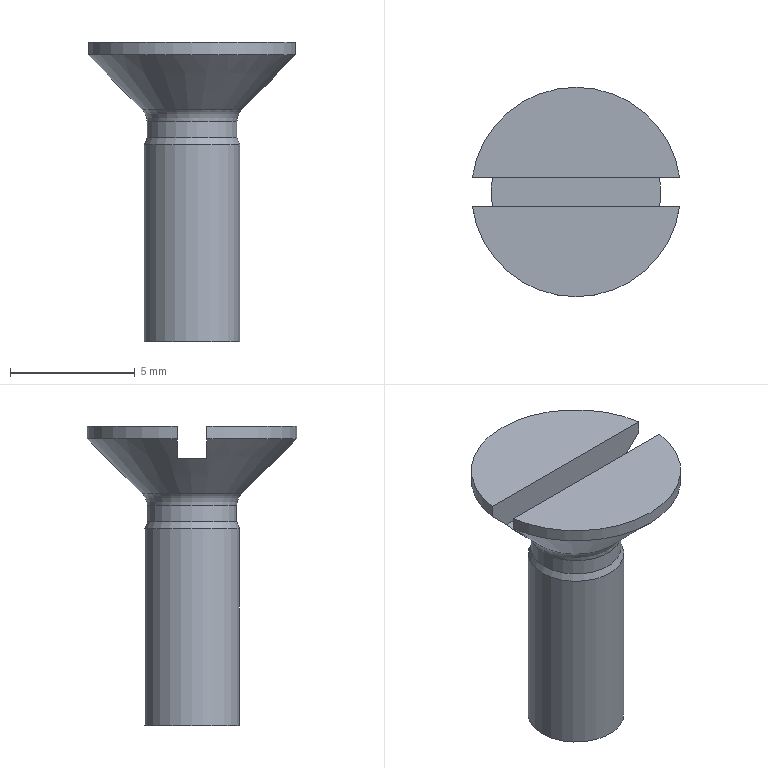Part | NX | features DATUM_CSYS 2, SKETCH 2, EXTRUDE 1, LINE 1, META 1, SWP104 1, SYMBOLIC_THREAD 1, THREADS 1 | 1 solid | 13 faces | box 8.314 x 8.4 x 12 mm | volume 190.86 mm3 | plane 6 | cylinder 4 | cone 2 | torus 1 | commonest cylinder face diameters 8.4 x2 3.61 x1 3.838 x1
STEP:
#1=CARTESIAN_POINT('',(4.157,0.6,0.));
#2=VERTEX_POINT('',#1);
#3=CARTESIAN_POINT('',(-4.157,0.6,0.));
#4=VERTEX_POINT('',#3);
#5=CARTESIAN_POINT('',(9.4,0.6,0.));
#6=DIRECTION('',(-1.,0.,0.));
#7=VECTOR('',#6,1000.);
#8=LINE('',#5,#7);
#9=EDGE_CURVE('',#2,#4,#8,.T.);
#10=ORIENTED_EDGE('',*,*,#9,.F.);
#11=CARTESIAN_POINT('',(0.,0.,0.));
#12=DIRECTION('',(0.,0.,-1.));
#13=DIRECTION('',(-1.,0.,0.));
#14=AXIS2_PLACEMENT_3D('',#11,#12,#13);
#15=CIRCLE('',#14,4.2);
#16=EDGE_CURVE('',#4,#2,#15,.T.);
#17=ORIENTED_EDGE('',*,*,#16,.F.);
#18=EDGE_LOOP('',(#10,#17));
#19=FACE_BOUND('',#18,.T.);
#20=CARTESIAN_POINT('',(0.,0.,0.));
#21=DIRECTION('',(0.,0.,-1.));
#22=DIRECTION('',(-1.,0.,0.));
#23=AXIS2_PLACEMENT_3D('',#20,#21,#22);
#24=PLANE('',#23);
#25=ADVANCED_FACE('',(#19),#24,.F.);
#26=ORIENTED_EDGE('',*,*,#16,.T.);
#27=CARTESIAN_POINT('',(4.157,0.6,-0.5));
#28=VERTEX_POINT('',#27);
#29=CARTESIAN_POINT('',(4.157,0.6,0.));
#30=DIRECTION('',(0.,0.,-1.));
#31=VECTOR('',#30,1000.);
#32=LINE('',#29,#31);
#33=EDGE_CURVE('',#2,#28,#32,.T.);
#34=ORIENTED_EDGE('',*,*,#33,.T.);
#35=CARTESIAN_POINT('',(-4.157,0.6,-0.5));
#36=VERTEX_POINT('',#35);
#37=CARTESIAN_POINT('',(0.,0.,-0.5));
#38=DIRECTION('',(0.,0.,-1.));
#39=DIRECTION('',(-1.,0.,0.));
#40=AXIS2_PLACEMENT_3D('',#37,#38,#39);
#41=CIRCLE('',#40,4.2);
#42=EDGE_CURVE('',#36,#28,#41,.T.);
#43=ORIENTED_EDGE('',*,*,#42,.F.);
#44=CARTESIAN_POINT('',(-4.157,0.6,0.));
#45=DIRECTION('',(0.,0.,-1.));
#46=VECTOR('',#45,1000.);
#47=LINE('',#44,#46);
#48=EDGE_CURVE('',#36,#4,#47,.F.);
#49=ORIENTED_EDGE('',*,*,#48,.T.);
#50=EDGE_LOOP('',(#26,#34,#43,#49));
#51=FACE_BOUND('',#50,.T.);
#52=CARTESIAN_POINT('',(0.,0.,0.));
#53=DIRECTION('',(0.,0.,-1.));
#54=DIRECTION('',(-1.,0.,0.));
#55=AXIS2_PLACEMENT_3D('',#52,#53,#54);
#56=CYLINDRICAL_SURFACE('',#55,4.2);
#57=ADVANCED_FACE('',(#51),#56,.T.);
#58=CARTESIAN_POINT('',(-1.919,0.,-4.1));
#59=VERTEX_POINT('',#58);
#60=CARTESIAN_POINT('',(0.,0.,-4.1));
#61=DIRECTION('',(0.,0.,-1.));
#62=DIRECTION('',(-1.,0.,0.));
#63=AXIS2_PLACEMENT_3D('',#60,#61,#62);
#64=CIRCLE('',#63,1.919);
#65=EDGE_CURVE('',#59,#59,#64,.T.);
#66=ORIENTED_EDGE('',*,*,#65,.F.);
#67=EDGE_LOOP('',(#66));
#68=FACE_BOUND('',#67,.T.);
#69=CARTESIAN_POINT('',(-1.805,0.,-3.82));
#70=VERTEX_POINT('',#69);
#71=CARTESIAN_POINT('',(0.,0.,-3.82));
#72=DIRECTION('',(0.,0.,-1.));
#73=DIRECTION('',(-1.,0.,0.));
#74=AXIS2_PLACEMENT_3D('',#71,#72,#73);
#75=CIRCLE('',#74,1.805);
#76=EDGE_CURVE('',#70,#70,#75,.T.);
#77=ORIENTED_EDGE('',*,*,#76,.T.);
#78=EDGE_LOOP('',(#77));
#79=FACE_BOUND('',#78,.T.);
#80=CARTESIAN_POINT('',(0.,0.,-3.82));
#81=DIRECTION('',(0.,0.,-1.));
#82=DIRECTION('',(-1.,0.,0.));
#83=AXIS2_PLACEMENT_3D('',#80,#81,#82);
#84=CONICAL_SURFACE('',#83,1.805,0.3866);
#85=ADVANCED_FACE('',(#68,#79),#84,.T.);
#86=CARTESIAN_POINT('',(-1.919,0.,-12.));
#87=VERTEX_POINT('',#86);
#88=CARTESIAN_POINT('',(0.,0.,-12.));
#89=DIRECTION('',(0.,0.,-1.));
#90=DIRECTION('',(-1.,0.,0.));
#91=AXIS2_PLACEMENT_3D('',#88,#89,#90);
#92=CIRCLE('',#91,1.919);
#93=EDGE_CURVE('',#87,#87,#92,.T.);
#94=ORIENTED_EDGE('',*,*,#93,.F.);
#95=EDGE_LOOP('',(#94));
#96=FACE_BOUND('',#95,.T.);
#97=ORIENTED_EDGE('',*,*,#65,.T.);
#98=EDGE_LOOP('',(#97));
#99=FACE_BOUND('',#98,.T.);
#100=CARTESIAN_POINT('',(0.,0.,0.));
#101=DIRECTION('',(0.,0.,-1.));
#102=DIRECTION('',(-1.,0.,0.));
#103=AXIS2_PLACEMENT_3D('',#100,#101,#102);
#104=CYLINDRICAL_SURFACE('',#103,1.919);
#105=ADVANCED_FACE('',(#96,#99),#104,.T.);
#106=ORIENTED_EDGE('',*,*,#93,.T.);
#107=EDGE_LOOP('',(#106));
#108=FACE_BOUND('',#107,.T.);
#109=CARTESIAN_POINT('',(0.,1.919,-12.));
#110=DIRECTION('',(0.,0.,1.));
#111=DIRECTION('',(1.,0.,0.));
#112=AXIS2_PLACEMENT_3D('',#109,#110,#111);
#113=PLANE('',#112);
#114=ADVANCED_FACE('',(#108),#113,.F.);
#115=CARTESIAN_POINT('',(4.157,-0.6,0.));
#116=VERTEX_POINT('',#115);
#117=CARTESIAN_POINT('',(-4.157,-0.6,0.));
#118=VERTEX_POINT('',#117);
#119=CARTESIAN_POINT('',(0.,0.,0.));
#120=DIRECTION('',(0.,0.,-1.));
#121=DIRECTION('',(-1.,0.,0.));
#122=AXIS2_PLACEMENT_3D('',#119,#120,#121);
#123=CIRCLE('',#122,4.2);
#124=EDGE_CURVE('',#116,#118,#123,.T.);
#125=ORIENTED_EDGE('',*,*,#124,.F.);
#126=CARTESIAN_POINT('',(9.4,-0.6,0.));
#127=DIRECTION('',(-1.,0.,0.));
#128=VECTOR('',#127,1000.);
#129=LINE('',#126,#128);
#130=EDGE_CURVE('',#116,#118,#129,.T.);
#131=ORIENTED_EDGE('',*,*,#130,.T.);
#132=EDGE_LOOP('',(#125,#131));
#133=FACE_BOUND('',#132,.T.);
#134=CARTESIAN_POINT('',(0.,0.,0.));
#135=DIRECTION('',(0.,0.,-1.));
#136=DIRECTION('',(-1.,0.,0.));
#137=AXIS2_PLACEMENT_3D('',#134,#135,#136);
#138=PLANE('',#137);
#139=ADVANCED_FACE('',(#133),#138,.F.);
#140=ORIENTED_EDGE('',*,*,#124,.T.);
#141=CARTESIAN_POINT('',(-4.157,-0.6,-0.5));
#142=VERTEX_POINT('',#141);
#143=CARTESIAN_POINT('',(-4.157,-0.6,0.));
#144=DIRECTION('',(0.,0.,-1.));
#145=VECTOR('',#144,1000.);
#146=LINE('',#143,#145);
#147=EDGE_CURVE('',#118,#142,#146,.T.);
#148=ORIENTED_EDGE('',*,*,#147,.T.);
#149=CARTESIAN_POINT('',(4.157,-0.6,-0.5));
#150=VERTEX_POINT('',#149);
#151=CARTESIAN_POINT('',(0.,0.,-0.5));
#152=DIRECTION('',(0.,0.,-1.));
#153=DIRECTION('',(-1.,0.,0.));
#154=AXIS2_PLACEMENT_3D('',#151,#152,#153);
#155=CIRCLE('',#154,4.2);
#156=EDGE_CURVE('',#150,#142,#155,.T.);
#157=ORIENTED_EDGE('',*,*,#156,.F.);
#158=CARTESIAN_POINT('',(4.157,-0.6,0.));
#159=DIRECTION('',(0.,0.,-1.));
#160=VECTOR('',#159,1000.);
#161=LINE('',#158,#160);
#162=EDGE_CURVE('',#150,#116,#161,.F.);
#163=ORIENTED_EDGE('',*,*,#162,.T.);
#164=EDGE_LOOP('',(#140,#148,#157,#163));
#165=FACE_BOUND('',#164,.T.);
#166=CARTESIAN_POINT('',(0.,0.,0.));
#167=DIRECTION('',(0.,0.,-1.));
#168=DIRECTION('',(-1.,0.,0.));
#169=AXIS2_PLACEMENT_3D('',#166,#167,#168);
#170=CYLINDRICAL_SURFACE('',#169,4.2);
#171=ADVANCED_FACE('',(#165),#170,.T.);
#172=CARTESIAN_POINT('',(-2.,0.,-2.7));
#173=VERTEX_POINT('',#172);
#174=CARTESIAN_POINT('',(0.,0.,-2.7));
#175=DIRECTION('',(0.,0.,-1.));
#176=DIRECTION('',(-1.,0.,0.));
#177=AXIS2_PLACEMENT_3D('',#174,#175,#176);
#178=CIRCLE('',#177,2.);
#179=EDGE_CURVE('',#173,#173,#178,.T.);
#180=ORIENTED_EDGE('',*,*,#179,.F.);
#181=EDGE_LOOP('',(#180));
#182=FACE_BOUND('',#181,.T.);
#183=CARTESIAN_POINT('',(-3.347,-0.6,-1.3));
#184=VERTEX_POINT('',#183);
#185=CARTESIAN_POINT('',(-3.347,0.6,-1.3));
#186=VERTEX_POINT('',#185);
#187=CARTESIAN_POINT('',(0.,0.,-1.3));
#188=DIRECTION('',(0.,0.,-1.));
#189=DIRECTION('',(0.,1.,0.));
#190=AXIS2_PLACEMENT_3D('',#187,#188,#189);
#191=CIRCLE('',#190,3.4);
#192=EDGE_CURVE('',#184,#186,#191,.T.);
#193=ORIENTED_EDGE('',*,*,#192,.T.);
#194=CARTESIAN_POINT('',(-3.347,0.6,-1.3));
#195=CARTESIAN_POINT('',(-3.617,0.6,-1.034));
#196=CARTESIAN_POINT('',(-3.887,0.6,-0.767));
#197=CARTESIAN_POINT('',(-4.157,0.6,-0.5));
#198=B_SPLINE_CURVE_WITH_KNOTS('',3,(#194,#195,#196,#197),.UNSPECIFIED.,.F.,.F.,(4,4),(0.01717,0.01832),.UNSPECIFIED.);
#199=EDGE_CURVE('',#186,#36,#198,.T.);
#200=ORIENTED_EDGE('',*,*,#199,.T.);
#201=ORIENTED_EDGE('',*,*,#42,.T.);
#202=CARTESIAN_POINT('',(3.347,0.6,-1.3));
#203=VERTEX_POINT('',#202);
#204=CARTESIAN_POINT('',(4.157,0.6,-0.5));
#205=CARTESIAN_POINT('',(3.887,0.6,-0.767));
#206=CARTESIAN_POINT('',(3.617,0.6,-1.034));
#207=CARTESIAN_POINT('',(3.347,0.6,-1.3));
#208=B_SPLINE_CURVE_WITH_KNOTS('',3,(#204,#205,#206,#207),.UNSPECIFIED.,.F.,.F.,(4,4),(0.007177,0.008316),.UNSPECIFIED.);
#209=EDGE_CURVE('',#28,#203,#208,.T.);
#210=ORIENTED_EDGE('',*,*,#209,.T.);
#211=CARTESIAN_POINT('',(3.347,-0.6,-1.3));
#212=VERTEX_POINT('',#211);
#213=CARTESIAN_POINT('',(0.,0.,-1.3));
#214=DIRECTION('',(0.,0.,-1.));
#215=DIRECTION('',(0.,1.,0.));
#216=AXIS2_PLACEMENT_3D('',#213,#214,#215);
#217=CIRCLE('',#216,3.4);
#218=EDGE_CURVE('',#203,#212,#217,.T.);
#219=ORIENTED_EDGE('',*,*,#218,.T.);
#220=CARTESIAN_POINT('',(3.347,-0.6,-1.3));
#221=CARTESIAN_POINT('',(3.617,-0.6,-1.034));
#222=CARTESIAN_POINT('',(3.887,-0.6,-0.767));
#223=CARTESIAN_POINT('',(4.157,-0.6,-0.5));
#224=B_SPLINE_CURVE_WITH_KNOTS('',3,(#220,#221,#222,#223),.UNSPECIFIED.,.F.,.F.,(4,4),(0.01717,0.01832),.UNSPECIFIED.);
#225=EDGE_CURVE('',#212,#150,#224,.T.);
#226=ORIENTED_EDGE('',*,*,#225,.T.);
#227=ORIENTED_EDGE('',*,*,#156,.T.);
#228=CARTESIAN_POINT('',(-4.157,-0.6,-0.5));
#229=CARTESIAN_POINT('',(-3.887,-0.6,-0.767));
#230=CARTESIAN_POINT('',(-3.617,-0.6,-1.034));
#231=CARTESIAN_POINT('',(-3.347,-0.6,-1.3));
#232=B_SPLINE_CURVE_WITH_KNOTS('',3,(#228,#229,#230,#231),.UNSPECIFIED.,.F.,.F.,(4,4),(0.007177,0.008316),.UNSPECIFIED.);
#233=EDGE_CURVE('',#142,#184,#232,.T.);
#234=ORIENTED_EDGE('',*,*,#233,.T.);
#235=EDGE_LOOP('',(#193,#200,#201,#210,#219,#226,#227,#234));
#236=FACE_BOUND('',#235,.T.);
#237=CARTESIAN_POINT('',(0.,0.,-0.5));
#238=DIRECTION('',(0.,0.,1.));
#239=DIRECTION('',(1.,0.,0.));
#240=AXIS2_PLACEMENT_3D('',#237,#238,#239);
#241=CONICAL_SURFACE('',#240,4.2,0.7854);
#242=ADVANCED_FACE('',(#182,#236),#241,.T.);
#243=CARTESIAN_POINT('',(-1.805,0.,-3.171));
#244=VERTEX_POINT('',#243);
#245=CARTESIAN_POINT('',(0.,0.,-3.171));
#246=DIRECTION('',(0.,0.,-1.));
#247=DIRECTION('',(-1.,0.,0.));
#248=AXIS2_PLACEMENT_3D('',#245,#246,#247);
#249=CIRCLE('',#248,1.805);
#250=EDGE_CURVE('',#244,#244,#249,.T.);
#251=ORIENTED_EDGE('',*,*,#250,.F.);
#252=EDGE_LOOP('',(#251));
#253=FACE_BOUND('',#252,.T.);
#254=ORIENTED_EDGE('',*,*,#179,.T.);
#255=EDGE_LOOP('',(#254));
#256=FACE_BOUND('',#255,.T.);
#257=CARTESIAN_POINT('',(0.,0.,-3.171));
#258=DIRECTION('',(0.,0.,-1.));
#259=DIRECTION('',(-1.,0.,0.));
#260=AXIS2_PLACEMENT_3D('',#257,#258,#259);
#261=TOROIDAL_SURFACE('',#260,2.471,0.6658);
#262=ADVANCED_FACE('',(#253,#256),#261,.F.);
#263=ORIENTED_EDGE('',*,*,#76,.F.);
#264=EDGE_LOOP('',(#263));
#265=FACE_BOUND('',#264,.T.);
#266=ORIENTED_EDGE('',*,*,#250,.T.);
#267=EDGE_LOOP('',(#266));
#268=FACE_BOUND('',#267,.T.);
#269=CARTESIAN_POINT('',(0.,0.,0.));
#270=DIRECTION('',(0.,0.,-1.));
#271=DIRECTION('',(-1.,0.,0.));
#272=AXIS2_PLACEMENT_3D('',#269,#270,#271);
#273=CYLINDRICAL_SURFACE('',#272,1.805);
#274=ADVANCED_FACE('',(#265,#268),#273,.T.);
#275=ORIENTED_EDGE('',*,*,#9,.T.);
#276=ORIENTED_EDGE('',*,*,#48,.F.);
#277=ORIENTED_EDGE('',*,*,#199,.F.);
#278=CARTESIAN_POINT('',(9.4,0.6,-1.3));
#279=DIRECTION('',(-1.,0.,0.));
#280=VECTOR('',#279,1000.);
#281=LINE('',#278,#280);
#282=EDGE_CURVE('',#203,#186,#281,.T.);
#283=ORIENTED_EDGE('',*,*,#282,.F.);
#284=ORIENTED_EDGE('',*,*,#209,.F.);
#285=ORIENTED_EDGE('',*,*,#33,.F.);
#286=EDGE_LOOP('',(#275,#276,#277,#283,#284,#285));
#287=FACE_BOUND('',#286,.T.);
#288=CARTESIAN_POINT('',(9.4,0.6,0.));
#289=DIRECTION('',(0.,1.,0.));
#290=DIRECTION('',(0.,0.,1.));
#291=AXIS2_PLACEMENT_3D('',#288,#289,#290);
#292=PLANE('',#291);
#293=ADVANCED_FACE('',(#287),#292,.F.);
#294=ORIENTED_EDGE('',*,*,#282,.T.);
#295=ORIENTED_EDGE('',*,*,#192,.F.);
#296=CARTESIAN_POINT('',(9.4,-0.6,-1.3));
#297=DIRECTION('',(-1.,0.,0.));
#298=VECTOR('',#297,1000.);
#299=LINE('',#296,#298);
#300=EDGE_CURVE('',#212,#184,#299,.T.);
#301=ORIENTED_EDGE('',*,*,#300,.F.);
#302=ORIENTED_EDGE('',*,*,#218,.F.);
#303=EDGE_LOOP('',(#294,#295,#301,#302));
#304=FACE_BOUND('',#303,.T.);
#305=CARTESIAN_POINT('',(9.4,0.,-1.3));
#306=DIRECTION('',(0.,0.,-1.));
#307=DIRECTION('',(0.,1.,0.));
#308=AXIS2_PLACEMENT_3D('',#305,#306,#307);
#309=PLANE('',#308);
#310=ADVANCED_FACE('',(#304),#309,.F.);
#311=ORIENTED_EDGE('',*,*,#130,.F.);
#312=ORIENTED_EDGE('',*,*,#162,.F.);
#313=ORIENTED_EDGE('',*,*,#225,.F.);
#314=ORIENTED_EDGE('',*,*,#300,.T.);
#315=ORIENTED_EDGE('',*,*,#233,.F.);
#316=ORIENTED_EDGE('',*,*,#147,.F.);
#317=EDGE_LOOP('',(#311,#312,#313,#314,#315,#316));
#318=FACE_BOUND('',#317,.T.);
#319=CARTESIAN_POINT('',(9.4,-0.6,-1.3));
#320=DIRECTION('',(0.,-1.,0.));
#321=DIRECTION('',(0.,0.,-1.));
#322=AXIS2_PLACEMENT_3D('',#319,#320,#321);
#323=PLANE('',#322);
#324=ADVANCED_FACE('',(#318),#323,.F.);
#325=CLOSED_SHELL('',(#25,#57,#85,#105,#114,#139,#171,#242,#262,#274,#293,#310,#324));
#326=MANIFOLD_SOLID_BREP('',#325);
#327=(LENGTH_UNIT()NAMED_UNIT(*)SI_UNIT(.MILLI.,.METRE.));
#328=UNCERTAINTY_MEASURE_WITH_UNIT(LENGTH_MEASURE(0.0508),#327,'','');
#329=(NAMED_UNIT(*)PLANE_ANGLE_UNIT()SI_UNIT($,.RADIAN.));
#330=(NAMED_UNIT(*)SI_UNIT($,.STERADIAN.)SOLID_ANGLE_UNIT());
#331=(GEOMETRIC_REPRESENTATION_CONTEXT(3)GLOBAL_UNCERTAINTY_ASSIGNED_CONTEXT((#328))GLOBAL_UNIT_ASSIGNED_CONTEXT((#327,#329,#330))REPRESENTATION_CONTEXT('',''));
#332=ADVANCED_BREP_SHAPE_REPRESENTATION('',(#326),#331);